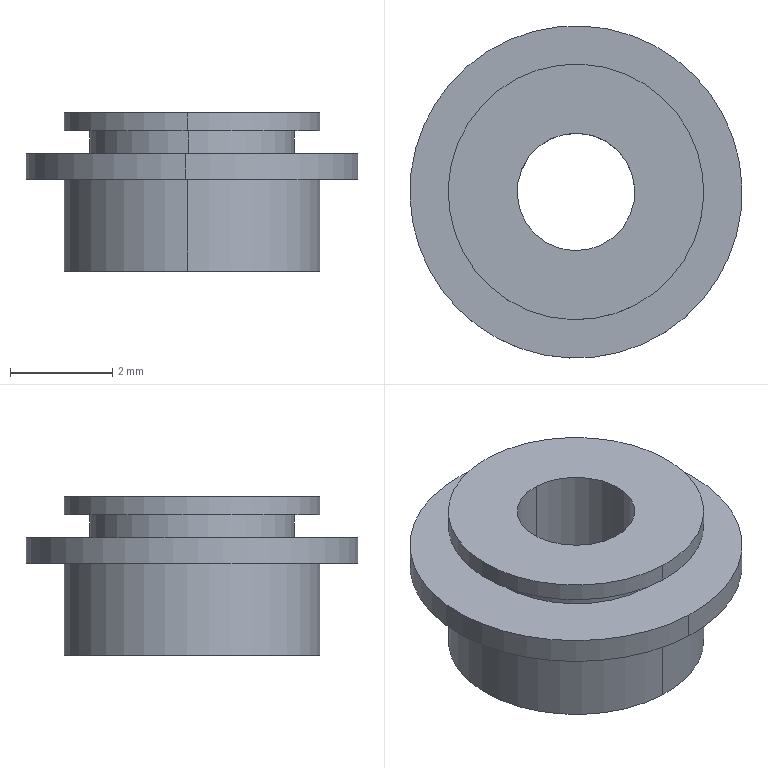Part | NX | features solid 2 | 1 solid | 17 faces | box 6.5 x 6.5 x 3.1 mm | volume 50.055 mm3 | cylinder 10 | plane 5 | cone 2 | commonest cylinder face diameters 5 x4 2.3 x2 4 x2 6.5 x2
STEP:
#1=CARTESIAN_POINT('',(-250.903,2147.128,6.2));
#2=VERTEX_POINT('',#1);
#3=CARTESIAN_POINT('',(-251.097,2142.132,6.2));
#4=VERTEX_POINT('',#3);
#5=CARTESIAN_POINT('',(-251.,2144.63,6.2));
#6=DIRECTION('',(0.,0.,-1.));
#7=DIRECTION('',(0.03897,0.9992,0.));
#8=AXIS2_PLACEMENT_3D('',#5,#6,#7);
#9=CIRCLE('',#8,2.5);
#10=EDGE_CURVE('',#2,#4,#9,.T.);
#11=ORIENTED_EDGE('',*,*,#10,.T.);
#12=CARTESIAN_POINT('',(-251.,2144.63,6.2));
#13=DIRECTION('',(0.,0.,-1.));
#14=DIRECTION('',(-0.03897,-0.9992,0.));
#15=AXIS2_PLACEMENT_3D('',#12,#13,#14);
#16=CIRCLE('',#15,2.5);
#17=EDGE_CURVE('',#4,#2,#16,.T.);
#18=ORIENTED_EDGE('',*,*,#17,.T.);
#19=EDGE_LOOP('',(#11,#18));
#20=FACE_BOUND('',#19,.T.);
#21=CARTESIAN_POINT('',(-250.932,2146.379,6.2));
#22=VERTEX_POINT('',#21);
#23=CARTESIAN_POINT('',(-251.068,2142.881,6.2));
#24=VERTEX_POINT('',#23);
#25=CARTESIAN_POINT('',(-251.,2144.63,6.2));
#26=DIRECTION('',(0.,0.,1.));
#27=DIRECTION('',(0.03897,0.9992,0.));
#28=AXIS2_PLACEMENT_3D('',#25,#26,#27);
#29=CIRCLE('',#28,1.75);
#30=EDGE_CURVE('',#22,#24,#29,.T.);
#31=ORIENTED_EDGE('',*,*,#30,.T.);
#32=CARTESIAN_POINT('',(-251.,2144.63,6.2));
#33=DIRECTION('',(0.,0.,1.));
#34=DIRECTION('',(-0.03897,-0.9992,0.));
#35=AXIS2_PLACEMENT_3D('',#32,#33,#34);
#36=CIRCLE('',#35,1.75);
#37=EDGE_CURVE('',#24,#22,#36,.T.);
#38=ORIENTED_EDGE('',*,*,#37,.T.);
#39=EDGE_LOOP('',(#31,#38));
#40=FACE_BOUND('',#39,.T.);
#41=CARTESIAN_POINT('',(-253.498,2144.727,6.2));
#42=DIRECTION('',(0.,0.,1.));
#43=DIRECTION('',(0.03897,0.9992,0.));
#44=AXIS2_PLACEMENT_3D('',#41,#42,#43);
#45=PLANE('',#44);
#46=ADVANCED_FACE('',(#20,#40),#45,.F.);
#47=CARTESIAN_POINT('',(-250.955,2145.779,6.8));
#48=VERTEX_POINT('',#47);
#49=CARTESIAN_POINT('',(-250.955,2145.779,6.8));
#50=DIRECTION('',(0.02756,0.7066,-0.7071));
#51=VECTOR('',#50,1000.);
#52=LINE('',#49,#51);
#53=EDGE_CURVE('',#48,#22,#52,.T.);
#54=ORIENTED_EDGE('',*,*,#53,.T.);
#55=ORIENTED_EDGE('',*,*,#37,.F.);
#56=CARTESIAN_POINT('',(-251.045,2143.481,6.8));
#57=VERTEX_POINT('',#56);
#58=CARTESIAN_POINT('',(-251.045,2143.481,6.8));
#59=DIRECTION('',(-0.02756,-0.7066,-0.7071));
#60=VECTOR('',#59,1000.);
#61=LINE('',#58,#60);
#62=EDGE_CURVE('',#24,#57,#61,.F.);
#63=ORIENTED_EDGE('',*,*,#62,.T.);
#64=CARTESIAN_POINT('',(-251.,2144.63,6.8));
#65=DIRECTION('',(0.,0.,1.));
#66=DIRECTION('',(-0.03897,-0.9992,0.));
#67=AXIS2_PLACEMENT_3D('',#64,#65,#66);
#68=CIRCLE('',#67,1.15);
#69=EDGE_CURVE('',#57,#48,#68,.T.);
#70=ORIENTED_EDGE('',*,*,#69,.T.);
#71=EDGE_LOOP('',(#54,#55,#63,#70));
#72=FACE_BOUND('',#71,.T.);
#73=CARTESIAN_POINT('',(-251.,2144.63,6.5));
#74=DIRECTION('',(0.,0.,-1.));
#75=DIRECTION('',(-0.03897,-0.9992,0.));
#76=AXIS2_PLACEMENT_3D('',#73,#74,#75);
#77=CONICAL_SURFACE('',#76,1.45,0.7854);
#78=ADVANCED_FACE('',(#72),#77,.F.);
#79=CARTESIAN_POINT('',(-250.955,2145.779,9.3));
#80=VERTEX_POINT('',#79);
#81=CARTESIAN_POINT('',(-250.955,2145.779,9.3));
#82=DIRECTION('',(0.,0.,-1.));
#83=VECTOR('',#82,1000.);
#84=LINE('',#81,#83);
#85=EDGE_CURVE('',#80,#48,#84,.T.);
#86=ORIENTED_EDGE('',*,*,#85,.T.);
#87=ORIENTED_EDGE('',*,*,#69,.F.);
#88=CARTESIAN_POINT('',(-251.045,2143.481,9.3));
#89=VERTEX_POINT('',#88);
#90=CARTESIAN_POINT('',(-251.045,2143.481,9.3));
#91=DIRECTION('',(0.,0.,-1.));
#92=VECTOR('',#91,1000.);
#93=LINE('',#90,#92);
#94=EDGE_CURVE('',#57,#89,#93,.F.);
#95=ORIENTED_EDGE('',*,*,#94,.T.);
#96=CARTESIAN_POINT('',(-251.,2144.63,9.3));
#97=DIRECTION('',(0.,0.,-1.));
#98=DIRECTION('',(0.03897,0.9992,0.));
#99=AXIS2_PLACEMENT_3D('',#96,#97,#98);
#100=CIRCLE('',#99,1.15);
#101=EDGE_CURVE('',#80,#89,#100,.T.);
#102=ORIENTED_EDGE('',*,*,#101,.F.);
#103=EDGE_LOOP('',(#86,#87,#95,#102));
#104=FACE_BOUND('',#103,.T.);
#105=CARTESIAN_POINT('',(-251.,2144.63,4.308));
#106=DIRECTION('',(0.,0.,-1.));
#107=DIRECTION('',(-0.03897,-0.9992,0.));
#108=AXIS2_PLACEMENT_3D('',#105,#106,#107);
#109=CYLINDRICAL_SURFACE('',#108,1.15);
#110=ADVANCED_FACE('',(#104),#109,.F.);
#111=CARTESIAN_POINT('',(-250.903,2147.128,9.3));
#112=VERTEX_POINT('',#111);
#113=CARTESIAN_POINT('',(-251.097,2142.132,9.3));
#114=VERTEX_POINT('',#113);
#115=CARTESIAN_POINT('',(-251.,2144.63,9.3));
#116=DIRECTION('',(0.,0.,1.));
#117=DIRECTION('',(0.03897,0.9992,0.));
#118=AXIS2_PLACEMENT_3D('',#115,#116,#117);
#119=CIRCLE('',#118,2.5);
#120=EDGE_CURVE('',#112,#114,#119,.T.);
#121=ORIENTED_EDGE('',*,*,#120,.T.);
#122=CARTESIAN_POINT('',(-251.,2144.63,9.3));
#123=DIRECTION('',(0.,0.,1.));
#124=DIRECTION('',(-0.03897,-0.9992,0.));
#125=AXIS2_PLACEMENT_3D('',#122,#123,#124);
#126=CIRCLE('',#125,2.5);
#127=EDGE_CURVE('',#114,#112,#126,.T.);
#128=ORIENTED_EDGE('',*,*,#127,.T.);
#129=EDGE_LOOP('',(#121,#128));
#130=FACE_BOUND('',#129,.T.);
#131=ORIENTED_EDGE('',*,*,#101,.T.);
#132=CARTESIAN_POINT('',(-251.,2144.63,9.3));
#133=DIRECTION('',(0.,0.,-1.));
#134=DIRECTION('',(-0.03897,-0.9992,0.));
#135=AXIS2_PLACEMENT_3D('',#132,#133,#134);
#136=CIRCLE('',#135,1.15);
#137=EDGE_CURVE('',#89,#80,#136,.T.);
#138=ORIENTED_EDGE('',*,*,#137,.T.);
#139=EDGE_LOOP('',(#131,#138));
#140=FACE_BOUND('',#139,.T.);
#141=CARTESIAN_POINT('',(-252.249,2144.679,9.3));
#142=DIRECTION('',(0.,0.,-1.));
#143=DIRECTION('',(-0.03897,-0.9992,0.));
#144=AXIS2_PLACEMENT_3D('',#141,#142,#143);
#145=PLANE('',#144);
#146=ADVANCED_FACE('',(#130,#140),#145,.F.);
#147=CARTESIAN_POINT('',(-250.903,2147.128,8.95));
#148=VERTEX_POINT('',#147);
#149=CARTESIAN_POINT('',(-250.903,2147.128,9.3));
#150=DIRECTION('',(0.,0.,-1.));
#151=VECTOR('',#150,1000.);
#152=LINE('',#149,#151);
#153=EDGE_CURVE('',#148,#112,#152,.F.);
#154=ORIENTED_EDGE('',*,*,#153,.T.);
#155=ORIENTED_EDGE('',*,*,#127,.F.);
#156=CARTESIAN_POINT('',(-251.097,2142.132,8.95));
#157=VERTEX_POINT('',#156);
#158=CARTESIAN_POINT('',(-251.097,2142.132,9.3));
#159=DIRECTION('',(0.,0.,-1.));
#160=VECTOR('',#159,1000.);
#161=LINE('',#158,#160);
#162=EDGE_CURVE('',#114,#157,#161,.T.);
#163=ORIENTED_EDGE('',*,*,#162,.T.);
#164=CARTESIAN_POINT('',(-251.,2144.63,8.95));
#165=DIRECTION('',(0.,0.,-1.));
#166=DIRECTION('',(0.03897,0.9992,0.));
#167=AXIS2_PLACEMENT_3D('',#164,#165,#166);
#168=CIRCLE('',#167,2.5);
#169=EDGE_CURVE('',#148,#157,#168,.T.);
#170=ORIENTED_EDGE('',*,*,#169,.F.);
#171=EDGE_LOOP('',(#154,#155,#163,#170));
#172=FACE_BOUND('',#171,.T.);
#173=CARTESIAN_POINT('',(-251.,2144.63,4.308));
#174=DIRECTION('',(0.,0.,-1.));
#175=DIRECTION('',(-0.03897,-0.9992,0.));
#176=AXIS2_PLACEMENT_3D('',#173,#174,#175);
#177=CYLINDRICAL_SURFACE('',#176,2.5);
#178=ADVANCED_FACE('',(#172),#177,.T.);
#179=ORIENTED_EDGE('',*,*,#169,.T.);
#180=CARTESIAN_POINT('',(-251.,2144.63,8.95));
#181=DIRECTION('',(0.,0.,-1.));
#182=DIRECTION('',(-0.03897,-0.9992,0.));
#183=AXIS2_PLACEMENT_3D('',#180,#181,#182);
#184=CIRCLE('',#183,2.5);
#185=EDGE_CURVE('',#157,#148,#184,.T.);
#186=ORIENTED_EDGE('',*,*,#185,.T.);
#187=EDGE_LOOP('',(#179,#186));
#188=FACE_BOUND('',#187,.T.);
#189=CARTESIAN_POINT('',(-250.922,2146.628,8.95));
#190=VERTEX_POINT('',#189);
#191=CARTESIAN_POINT('',(-251.078,2142.632,8.95));
#192=VERTEX_POINT('',#191);
#193=CARTESIAN_POINT('',(-251.,2144.63,8.95));
#194=DIRECTION('',(0.,0.,1.));
#195=DIRECTION('',(0.03897,0.9992,0.));
#196=AXIS2_PLACEMENT_3D('',#193,#194,#195);
#197=CIRCLE('',#196,2.);
#198=EDGE_CURVE('',#190,#192,#197,.T.);
#199=ORIENTED_EDGE('',*,*,#198,.T.);
#200=CARTESIAN_POINT('',(-251.,2144.63,8.95));
#201=DIRECTION('',(0.,0.,1.));
#202=DIRECTION('',(-0.03897,-0.9992,0.));
#203=AXIS2_PLACEMENT_3D('',#200,#201,#202);
#204=CIRCLE('',#203,2.);
#205=EDGE_CURVE('',#192,#190,#204,.T.);
#206=ORIENTED_EDGE('',*,*,#205,.T.);
#207=EDGE_LOOP('',(#199,#206));
#208=FACE_BOUND('',#207,.T.);
#209=CARTESIAN_POINT('',(-253.498,2144.727,8.95));
#210=DIRECTION('',(0.,0.,1.));
#211=DIRECTION('',(0.03897,0.9992,0.));
#212=AXIS2_PLACEMENT_3D('',#209,#210,#211);
#213=PLANE('',#212);
#214=ADVANCED_FACE('',(#188,#208),#213,.F.);
#215=CARTESIAN_POINT('',(-250.922,2146.628,8.5));
#216=VERTEX_POINT('',#215);
#217=CARTESIAN_POINT('',(-250.922,2146.628,8.95));
#218=DIRECTION('',(0.,0.,-1.));
#219=VECTOR('',#218,1000.);
#220=LINE('',#217,#219);
#221=EDGE_CURVE('',#190,#216,#220,.T.);
#222=ORIENTED_EDGE('',*,*,#221,.F.);
#223=ORIENTED_EDGE('',*,*,#205,.F.);
#224=CARTESIAN_POINT('',(-251.078,2142.632,8.5));
#225=VERTEX_POINT('',#224);
#226=CARTESIAN_POINT('',(-251.078,2142.632,8.95));
#227=DIRECTION('',(0.,0.,-1.));
#228=VECTOR('',#227,1000.);
#229=LINE('',#226,#228);
#230=EDGE_CURVE('',#225,#192,#229,.F.);
#231=ORIENTED_EDGE('',*,*,#230,.F.);
#232=CARTESIAN_POINT('',(-251.,2144.63,8.5));
#233=DIRECTION('',(0.,0.,-1.));
#234=DIRECTION('',(0.03897,0.9992,0.));
#235=AXIS2_PLACEMENT_3D('',#232,#233,#234);
#236=CIRCLE('',#235,2.);
#237=EDGE_CURVE('',#216,#225,#236,.T.);
#238=ORIENTED_EDGE('',*,*,#237,.F.);
#239=EDGE_LOOP('',(#222,#223,#231,#238));
#240=FACE_BOUND('',#239,.T.);
#241=CARTESIAN_POINT('',(-251.,2144.63,4.308));
#242=DIRECTION('',(0.,0.,-1.));
#243=DIRECTION('',(-0.03897,-0.9992,0.));
#244=AXIS2_PLACEMENT_3D('',#241,#242,#243);
#245=CYLINDRICAL_SURFACE('',#244,2.);
#246=ADVANCED_FACE('',(#240),#245,.T.);
#247=CARTESIAN_POINT('',(-250.873,2147.878,8.5));
#248=VERTEX_POINT('',#247);
#249=CARTESIAN_POINT('',(-251.127,2141.382,8.5));
#250=VERTEX_POINT('',#249);
#251=CARTESIAN_POINT('',(-251.,2144.63,8.5));
#252=DIRECTION('',(0.,0.,1.));
#253=DIRECTION('',(0.03897,0.9992,0.));
#254=AXIS2_PLACEMENT_3D('',#251,#252,#253);
#255=CIRCLE('',#254,3.25);
#256=EDGE_CURVE('',#248,#250,#255,.T.);
#257=ORIENTED_EDGE('',*,*,#256,.T.);
#258=CARTESIAN_POINT('',(-251.,2144.63,8.5));
#259=DIRECTION('',(0.,0.,1.));
#260=DIRECTION('',(-0.03897,-0.9992,0.));
#261=AXIS2_PLACEMENT_3D('',#258,#259,#260);
#262=CIRCLE('',#261,3.25);
#263=EDGE_CURVE('',#250,#248,#262,.T.);
#264=ORIENTED_EDGE('',*,*,#263,.T.);
#265=EDGE_LOOP('',(#257,#264));
#266=FACE_BOUND('',#265,.T.);
#267=ORIENTED_EDGE('',*,*,#237,.T.);
#268=CARTESIAN_POINT('',(-251.,2144.63,8.5));
#269=DIRECTION('',(0.,0.,-1.));
#270=DIRECTION('',(-0.03897,-0.9992,0.));
#271=AXIS2_PLACEMENT_3D('',#268,#269,#270);
#272=CIRCLE('',#271,2.);
#273=EDGE_CURVE('',#225,#216,#272,.T.);
#274=ORIENTED_EDGE('',*,*,#273,.T.);
#275=EDGE_LOOP('',(#267,#274));
#276=FACE_BOUND('',#275,.T.);
#277=CARTESIAN_POINT('',(-252.998,2144.708,8.5));
#278=DIRECTION('',(0.,0.,-1.));
#279=DIRECTION('',(-0.03897,-0.9992,0.));
#280=AXIS2_PLACEMENT_3D('',#277,#278,#279);
#281=PLANE('',#280);
#282=ADVANCED_FACE('',(#266,#276),#281,.F.);
#283=CARTESIAN_POINT('',(-250.873,2147.878,8.));
#284=VERTEX_POINT('',#283);
#285=CARTESIAN_POINT('',(-250.873,2147.878,8.5));
#286=DIRECTION('',(0.,0.,-1.));
#287=VECTOR('',#286,1000.);
#288=LINE('',#285,#287);
#289=EDGE_CURVE('',#284,#248,#288,.F.);
#290=ORIENTED_EDGE('',*,*,#289,.T.);
#291=ORIENTED_EDGE('',*,*,#263,.F.);
#292=CARTESIAN_POINT('',(-251.127,2141.382,8.));
#293=VERTEX_POINT('',#292);
#294=CARTESIAN_POINT('',(-251.127,2141.382,8.5));
#295=DIRECTION('',(0.,0.,-1.));
#296=VECTOR('',#295,1000.);
#297=LINE('',#294,#296);
#298=EDGE_CURVE('',#250,#293,#297,.T.);
#299=ORIENTED_EDGE('',*,*,#298,.T.);
#300=CARTESIAN_POINT('',(-251.,2144.63,8.));
#301=DIRECTION('',(0.,0.,-1.));
#302=DIRECTION('',(0.03897,0.9992,0.));
#303=AXIS2_PLACEMENT_3D('',#300,#301,#302);
#304=CIRCLE('',#303,3.25);
#305=EDGE_CURVE('',#284,#293,#304,.T.);
#306=ORIENTED_EDGE('',*,*,#305,.F.);
#307=EDGE_LOOP('',(#290,#291,#299,#306));
#308=FACE_BOUND('',#307,.T.);
#309=CARTESIAN_POINT('',(-251.,2144.63,4.308));
#310=DIRECTION('',(0.,0.,-1.));
#311=DIRECTION('',(-0.03897,-0.9992,0.));
#312=AXIS2_PLACEMENT_3D('',#309,#310,#311);
#313=CYLINDRICAL_SURFACE('',#312,3.25);
#314=ADVANCED_FACE('',(#308),#313,.T.);
#315=ORIENTED_EDGE('',*,*,#305,.T.);
#316=CARTESIAN_POINT('',(-251.,2144.63,8.));
#317=DIRECTION('',(0.,0.,-1.));
#318=DIRECTION('',(-0.03897,-0.9992,0.));
#319=AXIS2_PLACEMENT_3D('',#316,#317,#318);
#320=CIRCLE('',#319,3.25);
#321=EDGE_CURVE('',#293,#284,#320,.T.);
#322=ORIENTED_EDGE('',*,*,#321,.T.);
#323=EDGE_LOOP('',(#315,#322));
#324=FACE_BOUND('',#323,.T.);
#325=CARTESIAN_POINT('',(-250.903,2147.128,8.));
#326=VERTEX_POINT('',#325);
#327=CARTESIAN_POINT('',(-251.097,2142.132,8.));
#328=VERTEX_POINT('',#327);
#329=CARTESIAN_POINT('',(-251.,2144.63,8.));
#330=DIRECTION('',(0.,0.,1.));
#331=DIRECTION('',(0.03897,0.9992,0.));
#332=AXIS2_PLACEMENT_3D('',#329,#330,#331);
#333=CIRCLE('',#332,2.5);
#334=EDGE_CURVE('',#326,#328,#333,.T.);
#335=ORIENTED_EDGE('',*,*,#334,.T.);
#336=CARTESIAN_POINT('',(-251.,2144.63,8.));
#337=DIRECTION('',(0.,0.,1.));
#338=DIRECTION('',(-0.03897,-0.9992,0.));
#339=AXIS2_PLACEMENT_3D('',#336,#337,#338);
#340=CIRCLE('',#339,2.5);
#341=EDGE_CURVE('',#328,#326,#340,.T.);
#342=ORIENTED_EDGE('',*,*,#341,.T.);
#343=EDGE_LOOP('',(#335,#342));
#344=FACE_BOUND('',#343,.T.);
#345=CARTESIAN_POINT('',(-254.248,2144.757,8.));
#346=DIRECTION('',(0.,0.,1.));
#347=DIRECTION('',(0.03897,0.9992,0.));
#348=AXIS2_PLACEMENT_3D('',#345,#346,#347);
#349=PLANE('',#348);
#350=ADVANCED_FACE('',(#324,#344),#349,.F.);
#351=CARTESIAN_POINT('',(-250.903,2147.128,8.));
#352=DIRECTION('',(0.,0.,-1.));
#353=VECTOR('',#352,1000.);
#354=LINE('',#351,#353);
#355=EDGE_CURVE('',#326,#2,#354,.T.);
#356=ORIENTED_EDGE('',*,*,#355,.F.);
#357=ORIENTED_EDGE('',*,*,#341,.F.);
#358=CARTESIAN_POINT('',(-251.097,2142.132,8.));
#359=DIRECTION('',(0.,0.,-1.));
#360=VECTOR('',#359,1000.);
#361=LINE('',#358,#360);
#362=EDGE_CURVE('',#4,#328,#361,.F.);
#363=ORIENTED_EDGE('',*,*,#362,.F.);
#364=ORIENTED_EDGE('',*,*,#10,.F.);
#365=EDGE_LOOP('',(#356,#357,#363,#364));
#366=FACE_BOUND('',#365,.T.);
#367=CARTESIAN_POINT('',(-251.,2144.63,4.308));
#368=DIRECTION('',(0.,0.,-1.));
#369=DIRECTION('',(-0.03897,-0.9992,0.));
#370=AXIS2_PLACEMENT_3D('',#367,#368,#369);
#371=CYLINDRICAL_SURFACE('',#370,2.5);
#372=ADVANCED_FACE('',(#366),#371,.T.);
#373=ORIENTED_EDGE('',*,*,#362,.T.);
#374=ORIENTED_EDGE('',*,*,#334,.F.);
#375=ORIENTED_EDGE('',*,*,#355,.T.);
#376=ORIENTED_EDGE('',*,*,#17,.F.);
#377=EDGE_LOOP('',(#373,#374,#375,#376));
#378=FACE_BOUND('',#377,.T.);
#379=CARTESIAN_POINT('',(-251.,2144.63,4.308));
#380=DIRECTION('',(0.,0.,-1.));
#381=DIRECTION('',(-0.03897,-0.9992,0.));
#382=AXIS2_PLACEMENT_3D('',#379,#380,#381);
#383=CYLINDRICAL_SURFACE('',#382,2.5);
#384=ADVANCED_FACE('',(#378),#383,.T.);
#385=ORIENTED_EDGE('',*,*,#298,.F.);
#386=ORIENTED_EDGE('',*,*,#256,.F.);
#387=ORIENTED_EDGE('',*,*,#289,.F.);
#388=ORIENTED_EDGE('',*,*,#321,.F.);
#389=EDGE_LOOP('',(#385,#386,#387,#388));
#390=FACE_BOUND('',#389,.T.);
#391=CARTESIAN_POINT('',(-251.,2144.63,4.308));
#392=DIRECTION('',(0.,0.,-1.));
#393=DIRECTION('',(-0.03897,-0.9992,0.));
#394=AXIS2_PLACEMENT_3D('',#391,#392,#393);
#395=CYLINDRICAL_SURFACE('',#394,3.25);
#396=ADVANCED_FACE('',(#390),#395,.T.);
#397=ORIENTED_EDGE('',*,*,#230,.T.);
#398=ORIENTED_EDGE('',*,*,#198,.F.);
#399=ORIENTED_EDGE('',*,*,#221,.T.);
#400=ORIENTED_EDGE('',*,*,#273,.F.);
#401=EDGE_LOOP('',(#397,#398,#399,#400));
#402=FACE_BOUND('',#401,.T.);
#403=CARTESIAN_POINT('',(-251.,2144.63,4.308));
#404=DIRECTION('',(0.,0.,-1.));
#405=DIRECTION('',(-0.03897,-0.9992,0.));
#406=AXIS2_PLACEMENT_3D('',#403,#404,#405);
#407=CYLINDRICAL_SURFACE('',#406,2.);
#408=ADVANCED_FACE('',(#402),#407,.T.);
#409=ORIENTED_EDGE('',*,*,#162,.F.);
#410=ORIENTED_EDGE('',*,*,#120,.F.);
#411=ORIENTED_EDGE('',*,*,#153,.F.);
#412=ORIENTED_EDGE('',*,*,#185,.F.);
#413=EDGE_LOOP('',(#409,#410,#411,#412));
#414=FACE_BOUND('',#413,.T.);
#415=CARTESIAN_POINT('',(-251.,2144.63,4.308));
#416=DIRECTION('',(0.,0.,-1.));
#417=DIRECTION('',(-0.03897,-0.9992,0.));
#418=AXIS2_PLACEMENT_3D('',#415,#416,#417);
#419=CYLINDRICAL_SURFACE('',#418,2.5);
#420=ADVANCED_FACE('',(#414),#419,.T.);
#421=ORIENTED_EDGE('',*,*,#94,.F.);
#422=CARTESIAN_POINT('',(-251.,2144.63,6.8));
#423=DIRECTION('',(0.,0.,1.));
#424=DIRECTION('',(0.03897,0.9992,0.));
#425=AXIS2_PLACEMENT_3D('',#422,#423,#424);
#426=CIRCLE('',#425,1.15);
#427=EDGE_CURVE('',#48,#57,#426,.T.);
#428=ORIENTED_EDGE('',*,*,#427,.F.);
#429=ORIENTED_EDGE('',*,*,#85,.F.);
#430=ORIENTED_EDGE('',*,*,#137,.F.);
#431=EDGE_LOOP('',(#421,#428,#429,#430));
#432=FACE_BOUND('',#431,.T.);
#433=CARTESIAN_POINT('',(-251.,2144.63,4.308));
#434=DIRECTION('',(0.,0.,-1.));
#435=DIRECTION('',(-0.03897,-0.9992,0.));
#436=AXIS2_PLACEMENT_3D('',#433,#434,#435);
#437=CYLINDRICAL_SURFACE('',#436,1.15);
#438=ADVANCED_FACE('',(#432),#437,.F.);
#439=ORIENTED_EDGE('',*,*,#62,.F.);
#440=ORIENTED_EDGE('',*,*,#30,.F.);
#441=ORIENTED_EDGE('',*,*,#53,.F.);
#442=ORIENTED_EDGE('',*,*,#427,.T.);
#443=EDGE_LOOP('',(#439,#440,#441,#442));
#444=FACE_BOUND('',#443,.T.);
#445=CARTESIAN_POINT('',(-251.,2144.63,6.5));
#446=DIRECTION('',(0.,0.,-1.));
#447=DIRECTION('',(-0.03897,-0.9992,0.));
#448=AXIS2_PLACEMENT_3D('',#445,#446,#447);
#449=CONICAL_SURFACE('',#448,1.45,0.7854);
#450=ADVANCED_FACE('',(#444),#449,.F.);
#451=CLOSED_SHELL('',(#46,#78,#110,#146,#178,#214,#246,#282,#314,#350,#372,#384,#396,#408,#420,#438,#450));
#452=MANIFOLD_SOLID_BREP('',#451);
#453=(LENGTH_UNIT()NAMED_UNIT(*)SI_UNIT(.MILLI.,.METRE.));
#454=UNCERTAINTY_MEASURE_WITH_UNIT(LENGTH_MEASURE(0.00001),#453,'','');
#455=(NAMED_UNIT(*)PLANE_ANGLE_UNIT()SI_UNIT($,.RADIAN.));
#456=(NAMED_UNIT(*)SI_UNIT($,.STERADIAN.)SOLID_ANGLE_UNIT());
#457=(GEOMETRIC_REPRESENTATION_CONTEXT(3)GLOBAL_UNCERTAINTY_ASSIGNED_CONTEXT((#454))GLOBAL_UNIT_ASSIGNED_CONTEXT((#453,#455,#456))REPRESENTATION_CONTEXT('',''));
#458=ADVANCED_BREP_SHAPE_REPRESENTATION('',(#452),#457);